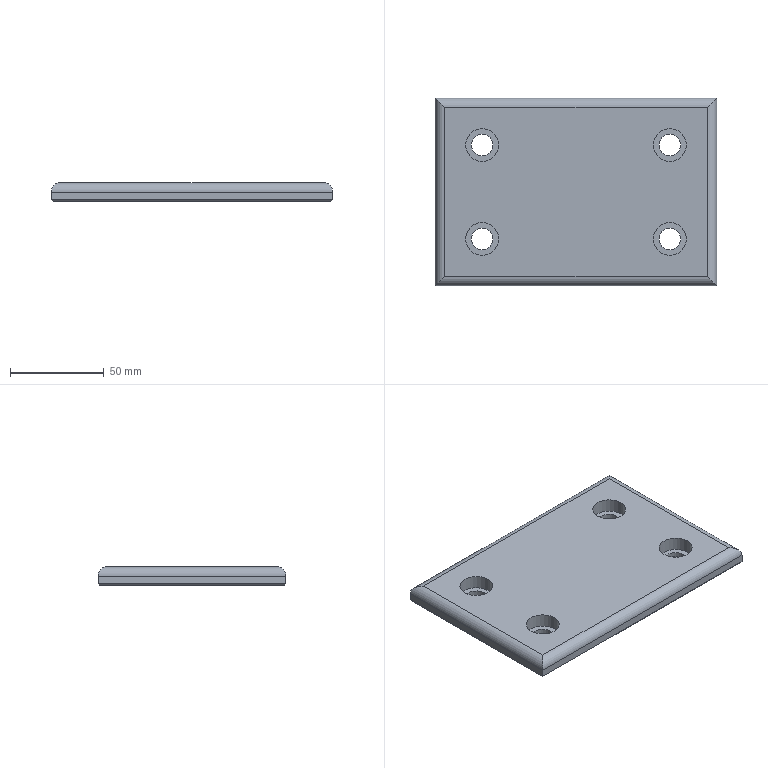Part | NX | features solid 2 | 1 solid | 26 faces | box 150 x 100 x 10 mm | volume 138972 mm3 | plane 14 | cylinder 12 | commonest cylinder face diameters 10 x4 11.5 x4 17.5 x4
STEP:
#1=CARTESIAN_POINT('',(-1090.,-730.,-129.));
#2=VERTEX_POINT('',#1);
#3=CARTESIAN_POINT('',(-1090.,-730.,-125.));
#4=VERTEX_POINT('',#3);
#5=CARTESIAN_POINT('',(-1090.,-730.,-130.));
#6=DIRECTION('',(0.,0.,1.));
#7=VECTOR('',#6,1000.);
#8=LINE('',#5,#7);
#9=EDGE_CURVE('',#2,#4,#8,.T.);
#10=ORIENTED_EDGE('',*,*,#9,.T.);
#11=CARTESIAN_POINT('',(-1090.,-630.,-125.));
#12=VERTEX_POINT('',#11);
#13=CARTESIAN_POINT('',(-1090.,-730.,-125.));
#14=DIRECTION('',(0.,-1.,0.));
#15=VECTOR('',#14,1000.);
#16=LINE('',#13,#15);
#17=EDGE_CURVE('',#12,#4,#16,.T.);
#18=ORIENTED_EDGE('',*,*,#17,.F.);
#19=CARTESIAN_POINT('',(-1090.,-630.,-129.));
#20=VERTEX_POINT('',#19);
#21=CARTESIAN_POINT('',(-1090.,-630.,-130.));
#22=DIRECTION('',(0.,0.,1.));
#23=VECTOR('',#22,1000.);
#24=LINE('',#21,#23);
#25=EDGE_CURVE('',#20,#12,#24,.T.);
#26=ORIENTED_EDGE('',*,*,#25,.F.);
#27=CARTESIAN_POINT('',(-1090.,-630.,-129.));
#28=DIRECTION('',(0.,1.,0.));
#29=VECTOR('',#28,1000.);
#30=LINE('',#27,#29);
#31=EDGE_CURVE('',#2,#20,#30,.T.);
#32=ORIENTED_EDGE('',*,*,#31,.F.);
#33=EDGE_LOOP('',(#10,#18,#26,#32));
#34=FACE_BOUND('',#33,.T.);
#35=CARTESIAN_POINT('',(-1090.,-630.,-130.));
#36=DIRECTION('',(1.,0.,0.));
#37=DIRECTION('',(0.,-1.,0.));
#38=AXIS2_PLACEMENT_3D('',#35,#36,#37);
#39=PLANE('',#38);
#40=ADVANCED_FACE('',(#34),#39,.F.);
#41=CARTESIAN_POINT('',(-940.,-730.,-129.));
#42=VERTEX_POINT('',#41);
#43=CARTESIAN_POINT('',(-940.,-730.,-125.));
#44=VERTEX_POINT('',#43);
#45=CARTESIAN_POINT('',(-940.,-730.,-130.));
#46=DIRECTION('',(0.,0.,1.));
#47=VECTOR('',#46,1000.);
#48=LINE('',#45,#47);
#49=EDGE_CURVE('',#42,#44,#48,.T.);
#50=ORIENTED_EDGE('',*,*,#49,.T.);
#51=CARTESIAN_POINT('',(-940.,-730.,-125.));
#52=DIRECTION('',(1.,0.,0.));
#53=VECTOR('',#52,1000.);
#54=LINE('',#51,#53);
#55=EDGE_CURVE('',#4,#44,#54,.T.);
#56=ORIENTED_EDGE('',*,*,#55,.F.);
#57=ORIENTED_EDGE('',*,*,#9,.F.);
#58=CARTESIAN_POINT('',(-1090.,-730.,-129.));
#59=DIRECTION('',(-1.,0.,0.));
#60=VECTOR('',#59,1000.);
#61=LINE('',#58,#60);
#62=EDGE_CURVE('',#42,#2,#61,.T.);
#63=ORIENTED_EDGE('',*,*,#62,.F.);
#64=EDGE_LOOP('',(#50,#56,#57,#63));
#65=FACE_BOUND('',#64,.T.);
#66=CARTESIAN_POINT('',(-1090.,-730.,-130.));
#67=DIRECTION('',(0.,1.,0.));
#68=DIRECTION('',(1.,0.,0.));
#69=AXIS2_PLACEMENT_3D('',#66,#67,#68);
#70=PLANE('',#69);
#71=ADVANCED_FACE('',(#65),#70,.F.);
#72=CARTESIAN_POINT('',(-940.,-630.,-129.));
#73=VERTEX_POINT('',#72);
#74=CARTESIAN_POINT('',(-940.,-630.,-125.));
#75=VERTEX_POINT('',#74);
#76=CARTESIAN_POINT('',(-940.,-630.,-130.));
#77=DIRECTION('',(0.,0.,1.));
#78=VECTOR('',#77,1000.);
#79=LINE('',#76,#78);
#80=EDGE_CURVE('',#73,#75,#79,.T.);
#81=ORIENTED_EDGE('',*,*,#80,.T.);
#82=CARTESIAN_POINT('',(-940.,-630.,-125.));
#83=DIRECTION('',(0.,1.,0.));
#84=VECTOR('',#83,1000.);
#85=LINE('',#82,#84);
#86=EDGE_CURVE('',#44,#75,#85,.T.);
#87=ORIENTED_EDGE('',*,*,#86,.F.);
#88=ORIENTED_EDGE('',*,*,#49,.F.);
#89=CARTESIAN_POINT('',(-940.,-730.,-129.));
#90=DIRECTION('',(0.,-1.,0.));
#91=VECTOR('',#90,1000.);
#92=LINE('',#89,#91);
#93=EDGE_CURVE('',#73,#42,#92,.T.);
#94=ORIENTED_EDGE('',*,*,#93,.F.);
#95=EDGE_LOOP('',(#81,#87,#88,#94));
#96=FACE_BOUND('',#95,.T.);
#97=CARTESIAN_POINT('',(-940.,-730.,-130.));
#98=DIRECTION('',(-1.,0.,0.));
#99=DIRECTION('',(0.,1.,0.));
#100=AXIS2_PLACEMENT_3D('',#97,#98,#99);
#101=PLANE('',#100);
#102=ADVANCED_FACE('',(#96),#101,.F.);
#103=ORIENTED_EDGE('',*,*,#25,.T.);
#104=CARTESIAN_POINT('',(-1090.,-630.,-125.));
#105=DIRECTION('',(-1.,0.,0.));
#106=VECTOR('',#105,1000.);
#107=LINE('',#104,#106);
#108=EDGE_CURVE('',#75,#12,#107,.T.);
#109=ORIENTED_EDGE('',*,*,#108,.F.);
#110=ORIENTED_EDGE('',*,*,#80,.F.);
#111=CARTESIAN_POINT('',(-940.,-630.,-129.));
#112=DIRECTION('',(1.,0.,0.));
#113=VECTOR('',#112,1000.);
#114=LINE('',#111,#113);
#115=EDGE_CURVE('',#20,#73,#114,.T.);
#116=ORIENTED_EDGE('',*,*,#115,.F.);
#117=EDGE_LOOP('',(#103,#109,#110,#116));
#118=FACE_BOUND('',#117,.T.);
#119=CARTESIAN_POINT('',(-940.,-630.,-130.));
#120=DIRECTION('',(0.,-1.,0.));
#121=DIRECTION('',(-1.,0.,0.));
#122=AXIS2_PLACEMENT_3D('',#119,#120,#121);
#123=PLANE('',#122);
#124=ADVANCED_FACE('',(#118),#123,.F.);
#125=CARTESIAN_POINT('',(-1089.,-631.,-130.));
#126=VERTEX_POINT('',#125);
#127=CARTESIAN_POINT('',(-1089.,-729.,-130.));
#128=VERTEX_POINT('',#127);
#129=CARTESIAN_POINT('',(-1089.,-630.,-130.));
#130=DIRECTION('',(0.,-1.,0.));
#131=VECTOR('',#130,1000.);
#132=LINE('',#129,#131);
#133=EDGE_CURVE('',#126,#128,#132,.T.);
#134=ORIENTED_EDGE('',*,*,#133,.F.);
#135=CARTESIAN_POINT('',(-941.,-631.,-130.));
#136=VERTEX_POINT('',#135);
#137=CARTESIAN_POINT('',(-1090.,-631.,-130.));
#138=DIRECTION('',(-1.,0.,0.));
#139=VECTOR('',#138,1000.);
#140=LINE('',#137,#139);
#141=EDGE_CURVE('',#136,#126,#140,.T.);
#142=ORIENTED_EDGE('',*,*,#141,.F.);
#143=CARTESIAN_POINT('',(-941.,-729.,-130.));
#144=VERTEX_POINT('',#143);
#145=CARTESIAN_POINT('',(-941.,-630.,-130.));
#146=DIRECTION('',(0.,1.,0.));
#147=VECTOR('',#146,1000.);
#148=LINE('',#145,#147);
#149=EDGE_CURVE('',#144,#136,#148,.T.);
#150=ORIENTED_EDGE('',*,*,#149,.F.);
#151=CARTESIAN_POINT('',(-1090.,-729.,-130.));
#152=DIRECTION('',(1.,0.,0.));
#153=VECTOR('',#152,1000.);
#154=LINE('',#151,#153);
#155=EDGE_CURVE('',#128,#144,#154,.T.);
#156=ORIENTED_EDGE('',*,*,#155,.F.);
#157=EDGE_LOOP('',(#134,#142,#150,#156));
#158=FACE_BOUND('',#157,.T.);
#159=CARTESIAN_POINT('',(-959.25,-655.,-130.));
#160=VERTEX_POINT('',#159);
#161=CARTESIAN_POINT('',(-965.,-655.,-130.));
#162=DIRECTION('',(0.,0.,-1.));
#163=DIRECTION('',(1.,0.,0.));
#164=AXIS2_PLACEMENT_3D('',#161,#162,#163);
#165=CIRCLE('',#164,5.75);
#166=EDGE_CURVE('',#160,#160,#165,.T.);
#167=ORIENTED_EDGE('',*,*,#166,.F.);
#168=EDGE_LOOP('',(#167));
#169=FACE_BOUND('',#168,.T.);
#170=CARTESIAN_POINT('',(-959.25,-705.,-130.));
#171=VERTEX_POINT('',#170);
#172=CARTESIAN_POINT('',(-965.,-705.,-130.));
#173=DIRECTION('',(0.,0.,-1.));
#174=DIRECTION('',(1.,0.,0.));
#175=AXIS2_PLACEMENT_3D('',#172,#173,#174);
#176=CIRCLE('',#175,5.75);
#177=EDGE_CURVE('',#171,#171,#176,.T.);
#178=ORIENTED_EDGE('',*,*,#177,.F.);
#179=EDGE_LOOP('',(#178));
#180=FACE_BOUND('',#179,.T.);
#181=CARTESIAN_POINT('',(-1059.25,-655.,-130.));
#182=VERTEX_POINT('',#181);
#183=CARTESIAN_POINT('',(-1065.,-655.,-130.));
#184=DIRECTION('',(0.,0.,-1.));
#185=DIRECTION('',(1.,0.,0.));
#186=AXIS2_PLACEMENT_3D('',#183,#184,#185);
#187=CIRCLE('',#186,5.75);
#188=EDGE_CURVE('',#182,#182,#187,.T.);
#189=ORIENTED_EDGE('',*,*,#188,.F.);
#190=EDGE_LOOP('',(#189));
#191=FACE_BOUND('',#190,.T.);
#192=CARTESIAN_POINT('',(-1059.25,-705.,-130.));
#193=VERTEX_POINT('',#192);
#194=CARTESIAN_POINT('',(-1065.,-705.,-130.));
#195=DIRECTION('',(0.,0.,-1.));
#196=DIRECTION('',(1.,0.,0.));
#197=AXIS2_PLACEMENT_3D('',#194,#195,#196);
#198=CIRCLE('',#197,5.75);
#199=EDGE_CURVE('',#193,#193,#198,.T.);
#200=ORIENTED_EDGE('',*,*,#199,.F.);
#201=EDGE_LOOP('',(#200));
#202=FACE_BOUND('',#201,.T.);
#203=CARTESIAN_POINT('',(-1090.,-630.,-130.));
#204=DIRECTION('',(0.,0.,1.));
#205=DIRECTION('',(1.,0.,0.));
#206=AXIS2_PLACEMENT_3D('',#203,#204,#205);
#207=PLANE('',#206);
#208=ADVANCED_FACE('',(#158,#169,#180,#191,#202),#207,.F.);
#209=CARTESIAN_POINT('',(-945.,-635.,-120.));
#210=VERTEX_POINT('',#209);
#211=CARTESIAN_POINT('',(-945.,-725.,-120.));
#212=VERTEX_POINT('',#211);
#213=CARTESIAN_POINT('',(-945.,-730.,-120.));
#214=DIRECTION('',(0.,1.,0.));
#215=VECTOR('',#214,1000.);
#216=LINE('',#213,#215);
#217=EDGE_CURVE('',#210,#212,#216,.F.);
#218=ORIENTED_EDGE('',*,*,#217,.F.);
#219=CARTESIAN_POINT('',(-1085.,-635.,-120.));
#220=VERTEX_POINT('',#219);
#221=CARTESIAN_POINT('',(-940.,-635.,-120.));
#222=DIRECTION('',(-1.,0.,0.));
#223=VECTOR('',#222,1000.);
#224=LINE('',#221,#223);
#225=EDGE_CURVE('',#220,#210,#224,.F.);
#226=ORIENTED_EDGE('',*,*,#225,.F.);
#227=CARTESIAN_POINT('',(-1085.,-725.,-120.));
#228=VERTEX_POINT('',#227);
#229=CARTESIAN_POINT('',(-1085.,-630.,-120.));
#230=DIRECTION('',(0.,-1.,0.));
#231=VECTOR('',#230,1000.);
#232=LINE('',#229,#231);
#233=EDGE_CURVE('',#228,#220,#232,.F.);
#234=ORIENTED_EDGE('',*,*,#233,.F.);
#235=CARTESIAN_POINT('',(-1090.,-725.,-120.));
#236=DIRECTION('',(1.,0.,0.));
#237=VECTOR('',#236,1000.);
#238=LINE('',#235,#237);
#239=EDGE_CURVE('',#212,#228,#238,.F.);
#240=ORIENTED_EDGE('',*,*,#239,.F.);
#241=EDGE_LOOP('',(#218,#226,#234,#240));
#242=FACE_BOUND('',#241,.T.);
#243=CARTESIAN_POINT('',(-973.75,-655.,-120.));
#244=VERTEX_POINT('',#243);
#245=CARTESIAN_POINT('',(-965.,-655.,-120.));
#246=DIRECTION('',(0.,0.,1.));
#247=DIRECTION('',(-1.,0.,0.));
#248=AXIS2_PLACEMENT_3D('',#245,#246,#247);
#249=CIRCLE('',#248,8.75);
#250=EDGE_CURVE('',#244,#244,#249,.T.);
#251=ORIENTED_EDGE('',*,*,#250,.F.);
#252=EDGE_LOOP('',(#251));
#253=FACE_BOUND('',#252,.T.);
#254=CARTESIAN_POINT('',(-973.75,-705.,-120.));
#255=VERTEX_POINT('',#254);
#256=CARTESIAN_POINT('',(-965.,-705.,-120.));
#257=DIRECTION('',(0.,0.,1.));
#258=DIRECTION('',(-1.,0.,0.));
#259=AXIS2_PLACEMENT_3D('',#256,#257,#258);
#260=CIRCLE('',#259,8.75);
#261=EDGE_CURVE('',#255,#255,#260,.T.);
#262=ORIENTED_EDGE('',*,*,#261,.F.);
#263=EDGE_LOOP('',(#262));
#264=FACE_BOUND('',#263,.T.);
#265=CARTESIAN_POINT('',(-1073.75,-655.,-120.));
#266=VERTEX_POINT('',#265);
#267=CARTESIAN_POINT('',(-1065.,-655.,-120.));
#268=DIRECTION('',(0.,0.,1.));
#269=DIRECTION('',(-1.,0.,0.));
#270=AXIS2_PLACEMENT_3D('',#267,#268,#269);
#271=CIRCLE('',#270,8.75);
#272=EDGE_CURVE('',#266,#266,#271,.T.);
#273=ORIENTED_EDGE('',*,*,#272,.F.);
#274=EDGE_LOOP('',(#273));
#275=FACE_BOUND('',#274,.T.);
#276=CARTESIAN_POINT('',(-1073.75,-705.,-120.));
#277=VERTEX_POINT('',#276);
#278=CARTESIAN_POINT('',(-1065.,-705.,-120.));
#279=DIRECTION('',(0.,0.,1.));
#280=DIRECTION('',(-1.,0.,0.));
#281=AXIS2_PLACEMENT_3D('',#278,#279,#280);
#282=CIRCLE('',#281,8.75);
#283=EDGE_CURVE('',#277,#277,#282,.T.);
#284=ORIENTED_EDGE('',*,*,#283,.F.);
#285=EDGE_LOOP('',(#284));
#286=FACE_BOUND('',#285,.T.);
#287=CARTESIAN_POINT('',(-1090.,-630.,-120.));
#288=DIRECTION('',(0.,0.,1.));
#289=DIRECTION('',(1.,0.,0.));
#290=AXIS2_PLACEMENT_3D('',#287,#288,#289);
#291=PLANE('',#290);
#292=ADVANCED_FACE('',(#242,#253,#264,#275,#286),#291,.T.);
#293=CARTESIAN_POINT('',(-1070.75,-705.,-127.3));
#294=VERTEX_POINT('',#293);
#295=CARTESIAN_POINT('',(-1065.,-705.,-127.3));
#296=DIRECTION('',(0.,0.,1.));
#297=DIRECTION('',(-1.,0.,0.));
#298=AXIS2_PLACEMENT_3D('',#295,#296,#297);
#299=CIRCLE('',#298,5.75);
#300=EDGE_CURVE('',#294,#294,#299,.T.);
#301=ORIENTED_EDGE('',*,*,#300,.T.);
#302=EDGE_LOOP('',(#301));
#303=FACE_BOUND('',#302,.T.);
#304=ORIENTED_EDGE('',*,*,#199,.T.);
#305=EDGE_LOOP('',(#304));
#306=FACE_BOUND('',#305,.T.);
#307=CARTESIAN_POINT('',(-1065.,-705.,-170.));
#308=DIRECTION('',(0.,0.,-1.));
#309=DIRECTION('',(-1.,0.,0.));
#310=AXIS2_PLACEMENT_3D('',#307,#308,#309);
#311=CYLINDRICAL_SURFACE('',#310,5.75);
#312=ADVANCED_FACE('',(#303,#306),#311,.F.);
#313=ORIENTED_EDGE('',*,*,#300,.F.);
#314=EDGE_LOOP('',(#313));
#315=FACE_BOUND('',#314,.T.);
#316=CARTESIAN_POINT('',(-1073.75,-705.,-127.3));
#317=VERTEX_POINT('',#316);
#318=CARTESIAN_POINT('',(-1065.,-705.,-127.3));
#319=DIRECTION('',(0.,0.,1.));
#320=DIRECTION('',(-1.,0.,0.));
#321=AXIS2_PLACEMENT_3D('',#318,#319,#320);
#322=CIRCLE('',#321,8.75);
#323=EDGE_CURVE('',#317,#317,#322,.T.);
#324=ORIENTED_EDGE('',*,*,#323,.T.);
#325=EDGE_LOOP('',(#324));
#326=FACE_BOUND('',#325,.T.);
#327=CARTESIAN_POINT('',(-1065.,-705.,-127.3));
#328=DIRECTION('',(0.,0.,-1.));
#329=DIRECTION('',(-1.,0.,0.));
#330=AXIS2_PLACEMENT_3D('',#327,#328,#329);
#331=PLANE('',#330);
#332=ADVANCED_FACE('',(#315,#326),#331,.F.);
#333=ORIENTED_EDGE('',*,*,#323,.F.);
#334=EDGE_LOOP('',(#333));
#335=FACE_BOUND('',#334,.T.);
#336=ORIENTED_EDGE('',*,*,#283,.T.);
#337=EDGE_LOOP('',(#336));
#338=FACE_BOUND('',#337,.T.);
#339=CARTESIAN_POINT('',(-1065.,-705.,-120.));
#340=DIRECTION('',(0.,0.,-1.));
#341=DIRECTION('',(-1.,0.,0.));
#342=AXIS2_PLACEMENT_3D('',#339,#340,#341);
#343=CYLINDRICAL_SURFACE('',#342,8.75);
#344=ADVANCED_FACE('',(#335,#338),#343,.F.);
#345=CARTESIAN_POINT('',(-1070.75,-655.,-127.3));
#346=VERTEX_POINT('',#345);
#347=CARTESIAN_POINT('',(-1065.,-655.,-127.3));
#348=DIRECTION('',(0.,0.,1.));
#349=DIRECTION('',(-1.,0.,0.));
#350=AXIS2_PLACEMENT_3D('',#347,#348,#349);
#351=CIRCLE('',#350,5.75);
#352=EDGE_CURVE('',#346,#346,#351,.T.);
#353=ORIENTED_EDGE('',*,*,#352,.T.);
#354=EDGE_LOOP('',(#353));
#355=FACE_BOUND('',#354,.T.);
#356=ORIENTED_EDGE('',*,*,#188,.T.);
#357=EDGE_LOOP('',(#356));
#358=FACE_BOUND('',#357,.T.);
#359=CARTESIAN_POINT('',(-1065.,-655.,-170.));
#360=DIRECTION('',(0.,0.,-1.));
#361=DIRECTION('',(-1.,0.,0.));
#362=AXIS2_PLACEMENT_3D('',#359,#360,#361);
#363=CYLINDRICAL_SURFACE('',#362,5.75);
#364=ADVANCED_FACE('',(#355,#358),#363,.F.);
#365=ORIENTED_EDGE('',*,*,#352,.F.);
#366=EDGE_LOOP('',(#365));
#367=FACE_BOUND('',#366,.T.);
#368=CARTESIAN_POINT('',(-1073.75,-655.,-127.3));
#369=VERTEX_POINT('',#368);
#370=CARTESIAN_POINT('',(-1065.,-655.,-127.3));
#371=DIRECTION('',(0.,0.,1.));
#372=DIRECTION('',(-1.,0.,0.));
#373=AXIS2_PLACEMENT_3D('',#370,#371,#372);
#374=CIRCLE('',#373,8.75);
#375=EDGE_CURVE('',#369,#369,#374,.T.);
#376=ORIENTED_EDGE('',*,*,#375,.T.);
#377=EDGE_LOOP('',(#376));
#378=FACE_BOUND('',#377,.T.);
#379=CARTESIAN_POINT('',(-1065.,-655.,-127.3));
#380=DIRECTION('',(0.,0.,-1.));
#381=DIRECTION('',(-1.,0.,0.));
#382=AXIS2_PLACEMENT_3D('',#379,#380,#381);
#383=PLANE('',#382);
#384=ADVANCED_FACE('',(#367,#378),#383,.F.);
#385=ORIENTED_EDGE('',*,*,#375,.F.);
#386=EDGE_LOOP('',(#385));
#387=FACE_BOUND('',#386,.T.);
#388=ORIENTED_EDGE('',*,*,#272,.T.);
#389=EDGE_LOOP('',(#388));
#390=FACE_BOUND('',#389,.T.);
#391=CARTESIAN_POINT('',(-1065.,-655.,-120.));
#392=DIRECTION('',(0.,0.,-1.));
#393=DIRECTION('',(-1.,0.,0.));
#394=AXIS2_PLACEMENT_3D('',#391,#392,#393);
#395=CYLINDRICAL_SURFACE('',#394,8.75);
#396=ADVANCED_FACE('',(#387,#390),#395,.F.);
#397=CARTESIAN_POINT('',(-970.75,-705.,-127.3));
#398=VERTEX_POINT('',#397);
#399=CARTESIAN_POINT('',(-965.,-705.,-127.3));
#400=DIRECTION('',(0.,0.,1.));
#401=DIRECTION('',(-1.,0.,0.));
#402=AXIS2_PLACEMENT_3D('',#399,#400,#401);
#403=CIRCLE('',#402,5.75);
#404=EDGE_CURVE('',#398,#398,#403,.T.);
#405=ORIENTED_EDGE('',*,*,#404,.T.);
#406=EDGE_LOOP('',(#405));
#407=FACE_BOUND('',#406,.T.);
#408=ORIENTED_EDGE('',*,*,#177,.T.);
#409=EDGE_LOOP('',(#408));
#410=FACE_BOUND('',#409,.T.);
#411=CARTESIAN_POINT('',(-965.,-705.,-170.));
#412=DIRECTION('',(0.,0.,-1.));
#413=DIRECTION('',(-1.,0.,0.));
#414=AXIS2_PLACEMENT_3D('',#411,#412,#413);
#415=CYLINDRICAL_SURFACE('',#414,5.75);
#416=ADVANCED_FACE('',(#407,#410),#415,.F.);
#417=ORIENTED_EDGE('',*,*,#404,.F.);
#418=EDGE_LOOP('',(#417));
#419=FACE_BOUND('',#418,.T.);
#420=CARTESIAN_POINT('',(-973.75,-705.,-127.3));
#421=VERTEX_POINT('',#420);
#422=CARTESIAN_POINT('',(-965.,-705.,-127.3));
#423=DIRECTION('',(0.,0.,1.));
#424=DIRECTION('',(-1.,0.,0.));
#425=AXIS2_PLACEMENT_3D('',#422,#423,#424);
#426=CIRCLE('',#425,8.75);
#427=EDGE_CURVE('',#421,#421,#426,.T.);
#428=ORIENTED_EDGE('',*,*,#427,.T.);
#429=EDGE_LOOP('',(#428));
#430=FACE_BOUND('',#429,.T.);
#431=CARTESIAN_POINT('',(-965.,-705.,-127.3));
#432=DIRECTION('',(0.,0.,-1.));
#433=DIRECTION('',(-1.,0.,0.));
#434=AXIS2_PLACEMENT_3D('',#431,#432,#433);
#435=PLANE('',#434);
#436=ADVANCED_FACE('',(#419,#430),#435,.F.);
#437=ORIENTED_EDGE('',*,*,#427,.F.);
#438=EDGE_LOOP('',(#437));
#439=FACE_BOUND('',#438,.T.);
#440=ORIENTED_EDGE('',*,*,#261,.T.);
#441=EDGE_LOOP('',(#440));
#442=FACE_BOUND('',#441,.T.);
#443=CARTESIAN_POINT('',(-965.,-705.,-120.));
#444=DIRECTION('',(0.,0.,-1.));
#445=DIRECTION('',(-1.,0.,0.));
#446=AXIS2_PLACEMENT_3D('',#443,#444,#445);
#447=CYLINDRICAL_SURFACE('',#446,8.75);
#448=ADVANCED_FACE('',(#439,#442),#447,.F.);
#449=CARTESIAN_POINT('',(-970.75,-655.,-127.3));
#450=VERTEX_POINT('',#449);
#451=CARTESIAN_POINT('',(-965.,-655.,-127.3));
#452=DIRECTION('',(0.,0.,1.));
#453=DIRECTION('',(-1.,0.,0.));
#454=AXIS2_PLACEMENT_3D('',#451,#452,#453);
#455=CIRCLE('',#454,5.75);
#456=EDGE_CURVE('',#450,#450,#455,.T.);
#457=ORIENTED_EDGE('',*,*,#456,.T.);
#458=EDGE_LOOP('',(#457));
#459=FACE_BOUND('',#458,.T.);
#460=ORIENTED_EDGE('',*,*,#166,.T.);
#461=EDGE_LOOP('',(#460));
#462=FACE_BOUND('',#461,.T.);
#463=CARTESIAN_POINT('',(-965.,-655.,-170.));
#464=DIRECTION('',(0.,0.,-1.));
#465=DIRECTION('',(-1.,0.,0.));
#466=AXIS2_PLACEMENT_3D('',#463,#464,#465);
#467=CYLINDRICAL_SURFACE('',#466,5.75);
#468=ADVANCED_FACE('',(#459,#462),#467,.F.);
#469=ORIENTED_EDGE('',*,*,#456,.F.);
#470=EDGE_LOOP('',(#469));
#471=FACE_BOUND('',#470,.T.);
#472=CARTESIAN_POINT('',(-973.75,-655.,-127.3));
#473=VERTEX_POINT('',#472);
#474=CARTESIAN_POINT('',(-965.,-655.,-127.3));
#475=DIRECTION('',(0.,0.,1.));
#476=DIRECTION('',(-1.,0.,0.));
#477=AXIS2_PLACEMENT_3D('',#474,#475,#476);
#478=CIRCLE('',#477,8.75);
#479=EDGE_CURVE('',#473,#473,#478,.T.);
#480=ORIENTED_EDGE('',*,*,#479,.T.);
#481=EDGE_LOOP('',(#480));
#482=FACE_BOUND('',#481,.T.);
#483=CARTESIAN_POINT('',(-965.,-655.,-127.3));
#484=DIRECTION('',(0.,0.,-1.));
#485=DIRECTION('',(-1.,0.,0.));
#486=AXIS2_PLACEMENT_3D('',#483,#484,#485);
#487=PLANE('',#486);
#488=ADVANCED_FACE('',(#471,#482),#487,.F.);
#489=ORIENTED_EDGE('',*,*,#479,.F.);
#490=EDGE_LOOP('',(#489));
#491=FACE_BOUND('',#490,.T.);
#492=ORIENTED_EDGE('',*,*,#250,.T.);
#493=EDGE_LOOP('',(#492));
#494=FACE_BOUND('',#493,.T.);
#495=CARTESIAN_POINT('',(-965.,-655.,-120.));
#496=DIRECTION('',(0.,0.,-1.));
#497=DIRECTION('',(-1.,0.,0.));
#498=AXIS2_PLACEMENT_3D('',#495,#496,#497);
#499=CYLINDRICAL_SURFACE('',#498,8.75);
#500=ADVANCED_FACE('',(#491,#494),#499,.F.);
#501=CARTESIAN_POINT('',(-945.,-635.,-125.));
#502=DIRECTION('',(-0.7071,0.7071,0.));
#503=DIRECTION('',(0.7071,0.7071,0.));
#504=AXIS2_PLACEMENT_3D('',#501,#502,#503);
#505=ELLIPSE('',#504,7.071,5.);
#506=EDGE_CURVE('',#210,#75,#505,.T.);
#507=ORIENTED_EDGE('',*,*,#506,.T.);
#508=ORIENTED_EDGE('',*,*,#108,.T.);
#509=CARTESIAN_POINT('',(-1085.,-635.,-125.));
#510=DIRECTION('',(-0.7071,-0.7071,0.));
#511=DIRECTION('',(-0.7071,0.7071,0.));
#512=AXIS2_PLACEMENT_3D('',#509,#510,#511);
#513=ELLIPSE('',#512,7.071,5.);
#514=EDGE_CURVE('',#12,#220,#513,.F.);
#515=ORIENTED_EDGE('',*,*,#514,.T.);
#516=ORIENTED_EDGE('',*,*,#225,.T.);
#517=EDGE_LOOP('',(#507,#508,#515,#516));
#518=FACE_BOUND('',#517,.T.);
#519=CARTESIAN_POINT('',(-940.,-635.,-125.));
#520=DIRECTION('',(1.,0.,0.));
#521=DIRECTION('',(0.,-1.,0.));
#522=AXIS2_PLACEMENT_3D('',#519,#520,#521);
#523=CYLINDRICAL_SURFACE('',#522,5.);
#524=ADVANCED_FACE('',(#518),#523,.T.);
#525=ORIENTED_EDGE('',*,*,#514,.F.);
#526=ORIENTED_EDGE('',*,*,#17,.T.);
#527=CARTESIAN_POINT('',(-1085.,-725.,-125.));
#528=DIRECTION('',(0.7071,-0.7071,0.));
#529=DIRECTION('',(0.7071,0.7071,0.));
#530=AXIS2_PLACEMENT_3D('',#527,#528,#529);
#531=ELLIPSE('',#530,7.071,5.);
#532=EDGE_CURVE('',#4,#228,#531,.F.);
#533=ORIENTED_EDGE('',*,*,#532,.T.);
#534=ORIENTED_EDGE('',*,*,#233,.T.);
#535=EDGE_LOOP('',(#525,#526,#533,#534));
#536=FACE_BOUND('',#535,.T.);
#537=CARTESIAN_POINT('',(-1085.,-630.,-125.));
#538=DIRECTION('',(0.,1.,0.));
#539=DIRECTION('',(1.,0.,0.));
#540=AXIS2_PLACEMENT_3D('',#537,#538,#539);
#541=CYLINDRICAL_SURFACE('',#540,5.);
#542=ADVANCED_FACE('',(#536),#541,.T.);
#543=ORIENTED_EDGE('',*,*,#506,.F.);
#544=ORIENTED_EDGE('',*,*,#217,.T.);
#545=CARTESIAN_POINT('',(-945.,-725.,-125.));
#546=DIRECTION('',(0.7071,0.7071,0.));
#547=DIRECTION('',(0.7071,-0.7071,0.));
#548=AXIS2_PLACEMENT_3D('',#545,#546,#547);
#549=ELLIPSE('',#548,7.071,5.);
#550=EDGE_CURVE('',#212,#44,#549,.T.);
#551=ORIENTED_EDGE('',*,*,#550,.T.);
#552=ORIENTED_EDGE('',*,*,#86,.T.);
#553=EDGE_LOOP('',(#543,#544,#551,#552));
#554=FACE_BOUND('',#553,.T.);
#555=CARTESIAN_POINT('',(-945.,-730.,-125.));
#556=DIRECTION('',(0.,-1.,0.));
#557=DIRECTION('',(-1.,0.,0.));
#558=AXIS2_PLACEMENT_3D('',#555,#556,#557);
#559=CYLINDRICAL_SURFACE('',#558,5.);
#560=ADVANCED_FACE('',(#554),#559,.T.);
#561=ORIENTED_EDGE('',*,*,#532,.F.);
#562=ORIENTED_EDGE('',*,*,#55,.T.);
#563=ORIENTED_EDGE('',*,*,#550,.F.);
#564=ORIENTED_EDGE('',*,*,#239,.T.);
#565=EDGE_LOOP('',(#561,#562,#563,#564));
#566=FACE_BOUND('',#565,.T.);
#567=CARTESIAN_POINT('',(-1090.,-725.,-125.));
#568=DIRECTION('',(-1.,0.,0.));
#569=DIRECTION('',(0.,1.,0.));
#570=AXIS2_PLACEMENT_3D('',#567,#568,#569);
#571=CYLINDRICAL_SURFACE('',#570,5.);
#572=ADVANCED_FACE('',(#566),#571,.T.);
#573=CARTESIAN_POINT('',(-990.667,-680.667,-179.667));
#574=DIRECTION('',(0.5774,0.5774,0.5774));
#575=VECTOR('',#574,1000.);
#576=LINE('',#573,#575);
#577=EDGE_CURVE('',#73,#136,#576,.F.);
#578=ORIENTED_EDGE('',*,*,#577,.T.);
#579=ORIENTED_EDGE('',*,*,#141,.T.);
#580=CARTESIAN_POINT('',(-1089.333,-630.667,-129.667));
#581=DIRECTION('',(-0.5774,0.5774,0.5774));
#582=VECTOR('',#581,1000.);
#583=LINE('',#580,#582);
#584=EDGE_CURVE('',#126,#20,#583,.T.);
#585=ORIENTED_EDGE('',*,*,#584,.T.);
#586=ORIENTED_EDGE('',*,*,#115,.T.);
#587=EDGE_LOOP('',(#578,#579,#585,#586));
#588=FACE_BOUND('',#587,.T.);
#589=CARTESIAN_POINT('',(-1090.,-631.,-130.));
#590=DIRECTION('',(0.,-0.7071,0.7071));
#591=DIRECTION('',(0.,0.7071,0.7071));
#592=AXIS2_PLACEMENT_3D('',#589,#590,#591);
#593=PLANE('',#592);
#594=ADVANCED_FACE('',(#588),#593,.F.);
#595=ORIENTED_EDGE('',*,*,#584,.F.);
#596=ORIENTED_EDGE('',*,*,#133,.T.);
#597=CARTESIAN_POINT('',(-1056.,-696.,-163.));
#598=DIRECTION('',(0.5774,0.5774,-0.5774));
#599=VECTOR('',#598,1000.);
#600=LINE('',#597,#599);
#601=EDGE_CURVE('',#128,#2,#600,.F.);
#602=ORIENTED_EDGE('',*,*,#601,.T.);
#603=ORIENTED_EDGE('',*,*,#31,.T.);
#604=EDGE_LOOP('',(#595,#596,#602,#603));
#605=FACE_BOUND('',#604,.T.);
#606=CARTESIAN_POINT('',(-1089.,-630.,-130.));
#607=DIRECTION('',(0.7071,0.,0.7071));
#608=DIRECTION('',(0.7071,0.,-0.7071));
#609=AXIS2_PLACEMENT_3D('',#606,#607,#608);
#610=PLANE('',#609);
#611=ADVANCED_FACE('',(#605),#610,.F.);
#612=ORIENTED_EDGE('',*,*,#577,.F.);
#613=ORIENTED_EDGE('',*,*,#93,.T.);
#614=CARTESIAN_POINT('',(-974.,-696.,-163.));
#615=DIRECTION('',(0.5774,-0.5774,0.5774));
#616=VECTOR('',#615,1000.);
#617=LINE('',#614,#616);
#618=EDGE_CURVE('',#42,#144,#617,.F.);
#619=ORIENTED_EDGE('',*,*,#618,.T.);
#620=ORIENTED_EDGE('',*,*,#149,.T.);
#621=EDGE_LOOP('',(#612,#613,#619,#620));
#622=FACE_BOUND('',#621,.T.);
#623=CARTESIAN_POINT('',(-941.,-630.,-130.));
#624=DIRECTION('',(-0.7071,0.,0.7071));
#625=DIRECTION('',(0.7071,0.,0.7071));
#626=AXIS2_PLACEMENT_3D('',#623,#624,#625);
#627=PLANE('',#626);
#628=ADVANCED_FACE('',(#622),#627,.F.);
#629=ORIENTED_EDGE('',*,*,#601,.F.);
#630=ORIENTED_EDGE('',*,*,#155,.T.);
#631=ORIENTED_EDGE('',*,*,#618,.F.);
#632=ORIENTED_EDGE('',*,*,#62,.T.);
#633=EDGE_LOOP('',(#629,#630,#631,#632));
#634=FACE_BOUND('',#633,.T.);
#635=CARTESIAN_POINT('',(-1090.,-729.,-130.));
#636=DIRECTION('',(0.,0.7071,0.7071));
#637=DIRECTION('',(0.,0.7071,-0.7071));
#638=AXIS2_PLACEMENT_3D('',#635,#636,#637);
#639=PLANE('',#638);
#640=ADVANCED_FACE('',(#634),#639,.F.);
#641=CLOSED_SHELL('',(#40,#71,#102,#124,#208,#292,#312,#332,#344,#364,#384,#396,#416,#436,#448,#468,#488,#500,#524,#542,#560,#572,#594,#611,#628,#640));
#642=MANIFOLD_SOLID_BREP('',#641);
#643=(LENGTH_UNIT()NAMED_UNIT(*)SI_UNIT(.MILLI.,.METRE.));
#644=UNCERTAINTY_MEASURE_WITH_UNIT(LENGTH_MEASURE(0.00001),#643,'','');
#645=(NAMED_UNIT(*)PLANE_ANGLE_UNIT()SI_UNIT($,.RADIAN.));
#646=(NAMED_UNIT(*)SI_UNIT($,.STERADIAN.)SOLID_ANGLE_UNIT());
#647=(GEOMETRIC_REPRESENTATION_CONTEXT(3)GLOBAL_UNCERTAINTY_ASSIGNED_CONTEXT((#644))GLOBAL_UNIT_ASSIGNED_CONTEXT((#643,#645,#646))REPRESENTATION_CONTEXT('',''));
#648=ADVANCED_BREP_SHAPE_REPRESENTATION('',(#642),#647);